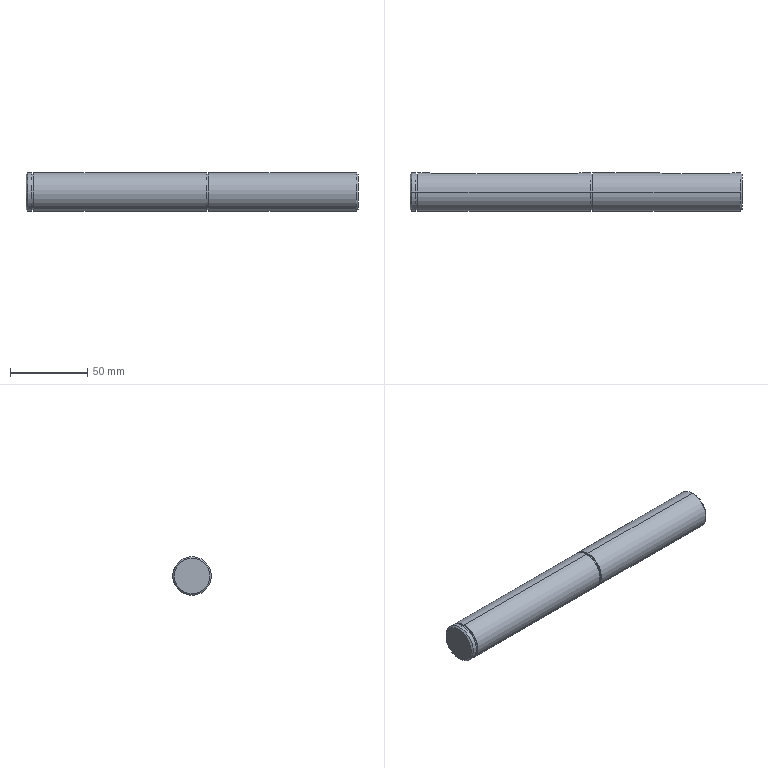Part | STEP file | 15-Roller drive shaft | 1 solid | 30 faces | box 215 x 25 x 25 mm | volume 100964 mm3 | cylinder 14 | plane 12 | cone 4 | commonest cylinder face diameters 25 x6 8 x4 23.2 x4